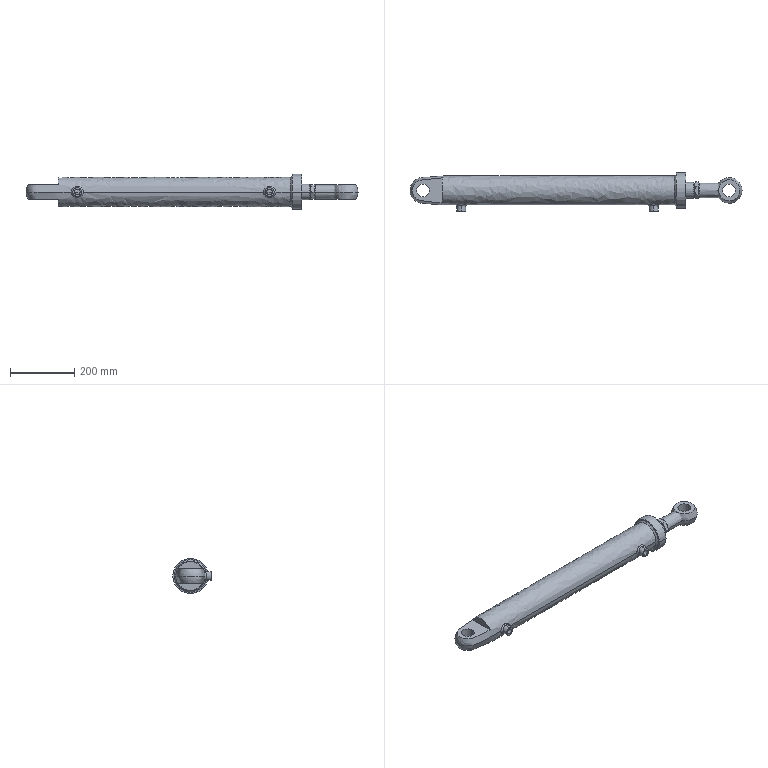Part | SolidWorks | 4 solids | 102 faces | box 1036 x 120 x 110 mm | volume 5671835 mm3 | plane 36 | cone 30 | cylinder 24 | spline 12 | commonest cylinder face diameters 30 x6 18 x4 28 x4 40 x4 50 x4 110 x2